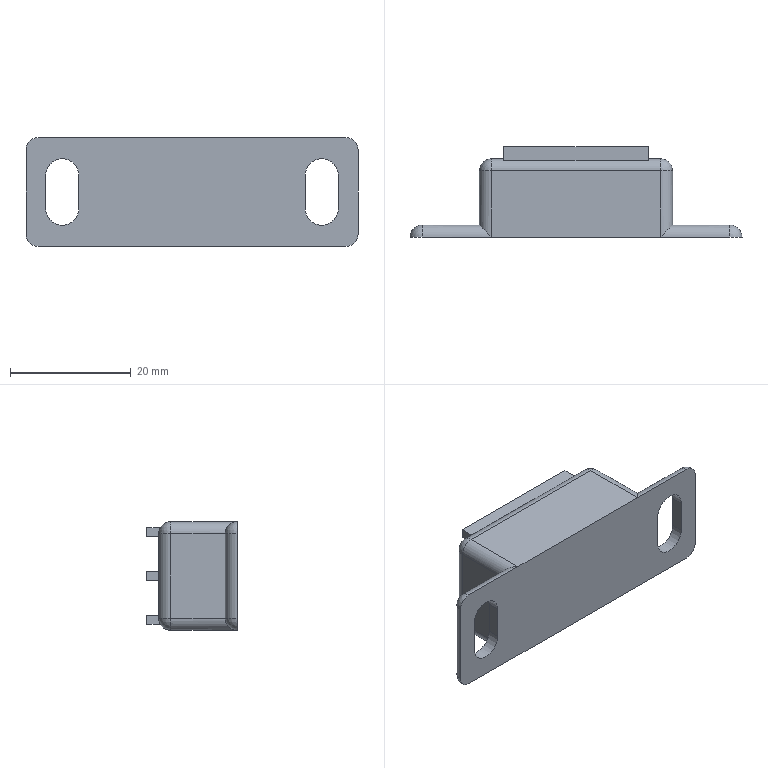Part | NX | features BREP 1 | 1 solid | 53 faces | box 55 x 15 x 18 mm | volume 8127 mm3 | plane 27 | cylinder 18 | sphere 8 | commonest cylinder face diameters 4 x14 5.5 x4
STEP:
#1=CARTESIAN_POINT('',(12.,13.,-6.5));
#2=VERTEX_POINT('',#1);
#3=CARTESIAN_POINT('',(12.,13.,-7.));
#4=VERTEX_POINT('',#3);
#5=CARTESIAN_POINT('',(12.,13.,9.));
#6=DIRECTION('',(0.,0.,-1.));
#7=VECTOR('',#6,1000.);
#8=LINE('',#5,#7);
#9=EDGE_CURVE('',#2,#4,#8,.T.);
#10=ORIENTED_EDGE('',*,*,#9,.F.);
#11=CARTESIAN_POINT('',(-12.,13.,-6.5));
#12=VERTEX_POINT('',#11);
#13=CARTESIAN_POINT('',(16.,13.,-6.5));
#14=DIRECTION('',(1.,0.,0.));
#15=VECTOR('',#14,1000.);
#16=LINE('',#13,#15);
#17=EDGE_CURVE('',#12,#2,#16,.T.);
#18=ORIENTED_EDGE('',*,*,#17,.F.);
#19=CARTESIAN_POINT('',(-12.,13.,-7.));
#20=VERTEX_POINT('',#19);
#21=CARTESIAN_POINT('',(-12.,13.,9.));
#22=DIRECTION('',(0.,0.,1.));
#23=VECTOR('',#22,1000.);
#24=LINE('',#21,#23);
#25=EDGE_CURVE('',#20,#12,#24,.T.);
#26=ORIENTED_EDGE('',*,*,#25,.F.);
#27=CARTESIAN_POINT('',(-14.,13.,-7.));
#28=VERTEX_POINT('',#27);
#29=CARTESIAN_POINT('',(16.,13.,-7.));
#30=DIRECTION('',(-1.,0.,0.));
#31=VECTOR('',#30,1000.);
#32=LINE('',#29,#31);
#33=EDGE_CURVE('',#20,#28,#32,.T.);
#34=ORIENTED_EDGE('',*,*,#33,.T.);
#35=CARTESIAN_POINT('',(-14.,13.,7.));
#36=VERTEX_POINT('',#35);
#37=CARTESIAN_POINT('',(-14.,13.,9.));
#38=DIRECTION('',(0.,0.,1.));
#39=VECTOR('',#38,1000.);
#40=LINE('',#37,#39);
#41=EDGE_CURVE('',#28,#36,#40,.T.);
#42=ORIENTED_EDGE('',*,*,#41,.T.);
#43=CARTESIAN_POINT('',(-12.,13.,7.));
#44=VERTEX_POINT('',#43);
#45=CARTESIAN_POINT('',(16.,13.,7.));
#46=DIRECTION('',(1.,0.,0.));
#47=VECTOR('',#46,1000.);
#48=LINE('',#45,#47);
#49=EDGE_CURVE('',#36,#44,#48,.T.);
#50=ORIENTED_EDGE('',*,*,#49,.T.);
#51=CARTESIAN_POINT('',(-12.,13.,6.5));
#52=VERTEX_POINT('',#51);
#53=CARTESIAN_POINT('',(-12.,13.,9.));
#54=DIRECTION('',(0.,0.,1.));
#55=VECTOR('',#54,1000.);
#56=LINE('',#53,#55);
#57=EDGE_CURVE('',#52,#44,#56,.T.);
#58=ORIENTED_EDGE('',*,*,#57,.F.);
#59=CARTESIAN_POINT('',(12.,13.,6.5));
#60=VERTEX_POINT('',#59);
#61=CARTESIAN_POINT('',(16.,13.,6.5));
#62=DIRECTION('',(-1.,0.,0.));
#63=VECTOR('',#62,1000.);
#64=LINE('',#61,#63);
#65=EDGE_CURVE('',#60,#52,#64,.T.);
#66=ORIENTED_EDGE('',*,*,#65,.F.);
#67=CARTESIAN_POINT('',(12.,13.,7.));
#68=VERTEX_POINT('',#67);
#69=CARTESIAN_POINT('',(12.,13.,9.));
#70=DIRECTION('',(0.,0.,-1.));
#71=VECTOR('',#70,1000.);
#72=LINE('',#69,#71);
#73=EDGE_CURVE('',#68,#60,#72,.T.);
#74=ORIENTED_EDGE('',*,*,#73,.F.);
#75=CARTESIAN_POINT('',(14.,13.,7.));
#76=VERTEX_POINT('',#75);
#77=CARTESIAN_POINT('',(16.,13.,7.));
#78=DIRECTION('',(1.,0.,0.));
#79=VECTOR('',#78,1000.);
#80=LINE('',#77,#79);
#81=EDGE_CURVE('',#68,#76,#80,.T.);
#82=ORIENTED_EDGE('',*,*,#81,.T.);
#83=CARTESIAN_POINT('',(14.,13.,-7.));
#84=VERTEX_POINT('',#83);
#85=CARTESIAN_POINT('',(14.,13.,9.));
#86=DIRECTION('',(0.,0.,-1.));
#87=VECTOR('',#86,1000.);
#88=LINE('',#85,#87);
#89=EDGE_CURVE('',#76,#84,#88,.T.);
#90=ORIENTED_EDGE('',*,*,#89,.T.);
#91=CARTESIAN_POINT('',(16.,13.,-7.));
#92=DIRECTION('',(-1.,0.,0.));
#93=VECTOR('',#92,1000.);
#94=LINE('',#91,#93);
#95=EDGE_CURVE('',#84,#4,#94,.T.);
#96=ORIENTED_EDGE('',*,*,#95,.T.);
#97=EDGE_LOOP('',(#10,#18,#26,#34,#42,#50,#58,#66,#74,#82,#90,#96));
#98=FACE_BOUND('',#97,.T.);
#99=CARTESIAN_POINT('',(12.,13.,0.75));
#100=VERTEX_POINT('',#99);
#101=CARTESIAN_POINT('',(12.,13.,-0.75));
#102=VERTEX_POINT('',#101);
#103=CARTESIAN_POINT('',(12.,13.,9.));
#104=DIRECTION('',(0.,0.,-1.));
#105=VECTOR('',#104,1000.);
#106=LINE('',#103,#105);
#107=EDGE_CURVE('',#100,#102,#106,.T.);
#108=ORIENTED_EDGE('',*,*,#107,.F.);
#109=CARTESIAN_POINT('',(-12.,13.,0.75));
#110=VERTEX_POINT('',#109);
#111=CARTESIAN_POINT('',(16.,13.,0.75));
#112=DIRECTION('',(1.,0.,0.));
#113=VECTOR('',#112,1000.);
#114=LINE('',#111,#113);
#115=EDGE_CURVE('',#110,#100,#114,.T.);
#116=ORIENTED_EDGE('',*,*,#115,.F.);
#117=CARTESIAN_POINT('',(-12.,13.,-0.75));
#118=VERTEX_POINT('',#117);
#119=CARTESIAN_POINT('',(-12.,13.,9.));
#120=DIRECTION('',(0.,0.,1.));
#121=VECTOR('',#120,1000.);
#122=LINE('',#119,#121);
#123=EDGE_CURVE('',#118,#110,#122,.T.);
#124=ORIENTED_EDGE('',*,*,#123,.F.);
#125=CARTESIAN_POINT('',(16.,13.,-0.75));
#126=DIRECTION('',(-1.,0.,0.));
#127=VECTOR('',#126,1000.);
#128=LINE('',#125,#127);
#129=EDGE_CURVE('',#102,#118,#128,.T.);
#130=ORIENTED_EDGE('',*,*,#129,.F.);
#131=EDGE_LOOP('',(#108,#116,#124,#130));
#132=FACE_BOUND('',#131,.T.);
#133=CARTESIAN_POINT('',(16.,13.,9.));
#134=DIRECTION('',(0.,-1.,0.));
#135=DIRECTION('',(0.,0.,-1.));
#136=AXIS2_PLACEMENT_3D('',#133,#134,#135);
#137=PLANE('',#136);
#138=ADVANCED_FACE('',(#98,#132),#137,.F.);
#139=CARTESIAN_POINT('',(-12.,12.732,-8.));
#140=VERTEX_POINT('',#139);
#141=CARTESIAN_POINT('',(12.,12.732,-8.));
#142=VERTEX_POINT('',#141);
#143=CARTESIAN_POINT('',(16.,12.732,-8.));
#144=DIRECTION('',(1.,0.,0.));
#145=VECTOR('',#144,1000.);
#146=LINE('',#143,#145);
#147=EDGE_CURVE('',#140,#142,#146,.T.);
#148=ORIENTED_EDGE('',*,*,#147,.T.);
#149=CARTESIAN_POINT('',(12.,11.,-7.));
#150=DIRECTION('',(1.,0.,0.));
#151=DIRECTION('',(0.,-1.,0.));
#152=AXIS2_PLACEMENT_3D('',#149,#150,#151);
#153=CIRCLE('',#152,2.);
#154=EDGE_CURVE('',#142,#4,#153,.T.);
#155=ORIENTED_EDGE('',*,*,#154,.T.);
#156=ORIENTED_EDGE('',*,*,#95,.F.);
#157=CARTESIAN_POINT('',(14.,11.,-9.));
#158=VERTEX_POINT('',#157);
#159=CARTESIAN_POINT('',(14.,11.,-7.));
#160=DIRECTION('',(1.,0.,0.));
#161=DIRECTION('',(0.,0.,-1.));
#162=AXIS2_PLACEMENT_3D('',#159,#160,#161);
#163=CIRCLE('',#162,2.);
#164=EDGE_CURVE('',#158,#84,#163,.T.);
#165=ORIENTED_EDGE('',*,*,#164,.F.);
#166=CARTESIAN_POINT('',(-14.,11.,-9.));
#167=VERTEX_POINT('',#166);
#168=CARTESIAN_POINT('',(0.,11.,-9.));
#169=DIRECTION('',(1.,0.,0.));
#170=VECTOR('',#169,1000.);
#171=LINE('',#168,#170);
#172=EDGE_CURVE('',#167,#158,#171,.T.);
#173=ORIENTED_EDGE('',*,*,#172,.F.);
#174=CARTESIAN_POINT('',(-14.,11.,-7.));
#175=DIRECTION('',(1.,0.,0.));
#176=DIRECTION('',(0.,0.,1.));
#177=AXIS2_PLACEMENT_3D('',#174,#175,#176);
#178=CIRCLE('',#177,2.);
#179=EDGE_CURVE('',#167,#28,#178,.T.);
#180=ORIENTED_EDGE('',*,*,#179,.T.);
#181=ORIENTED_EDGE('',*,*,#33,.F.);
#182=CARTESIAN_POINT('',(-12.,11.,-7.));
#183=DIRECTION('',(-1.,0.,0.));
#184=DIRECTION('',(0.,1.,0.));
#185=AXIS2_PLACEMENT_3D('',#182,#183,#184);
#186=CIRCLE('',#185,2.);
#187=EDGE_CURVE('',#20,#140,#186,.T.);
#188=ORIENTED_EDGE('',*,*,#187,.T.);
#189=EDGE_LOOP('',(#148,#155,#156,#165,#173,#180,#181,#188));
#190=FACE_BOUND('',#189,.T.);
#191=CARTESIAN_POINT('',(16.,11.,-7.));
#192=DIRECTION('',(-1.,0.,0.));
#193=DIRECTION('',(0.,-1.,0.));
#194=AXIS2_PLACEMENT_3D('',#191,#192,#193);
#195=CYLINDRICAL_SURFACE('',#194,2.);
#196=ADVANCED_FACE('',(#190),#195,.T.);
#197=ORIENTED_EDGE('',*,*,#81,.F.);
#198=CARTESIAN_POINT('',(12.,12.732,8.));
#199=VERTEX_POINT('',#198);
#200=CARTESIAN_POINT('',(12.,11.,7.));
#201=DIRECTION('',(1.,0.,0.));
#202=DIRECTION('',(0.,-1.,0.));
#203=AXIS2_PLACEMENT_3D('',#200,#201,#202);
#204=CIRCLE('',#203,2.);
#205=EDGE_CURVE('',#68,#199,#204,.T.);
#206=ORIENTED_EDGE('',*,*,#205,.T.);
#207=CARTESIAN_POINT('',(-12.,12.732,8.));
#208=VERTEX_POINT('',#207);
#209=CARTESIAN_POINT('',(0.,12.732,8.));
#210=DIRECTION('',(-1.,0.,0.));
#211=VECTOR('',#210,1000.);
#212=LINE('',#209,#211);
#213=EDGE_CURVE('',#199,#208,#212,.T.);
#214=ORIENTED_EDGE('',*,*,#213,.T.);
#215=CARTESIAN_POINT('',(-12.,11.,7.));
#216=DIRECTION('',(-1.,0.,0.));
#217=DIRECTION('',(0.,1.,0.));
#218=AXIS2_PLACEMENT_3D('',#215,#216,#217);
#219=CIRCLE('',#218,2.);
#220=EDGE_CURVE('',#208,#44,#219,.T.);
#221=ORIENTED_EDGE('',*,*,#220,.T.);
#222=ORIENTED_EDGE('',*,*,#49,.F.);
#223=CARTESIAN_POINT('',(-14.,11.,9.));
#224=VERTEX_POINT('',#223);
#225=CARTESIAN_POINT('',(-14.,11.,7.));
#226=DIRECTION('',(1.,0.,0.));
#227=DIRECTION('',(0.,0.,1.));
#228=AXIS2_PLACEMENT_3D('',#225,#226,#227);
#229=CIRCLE('',#228,2.);
#230=EDGE_CURVE('',#36,#224,#229,.T.);
#231=ORIENTED_EDGE('',*,*,#230,.T.);
#232=CARTESIAN_POINT('',(14.,11.,9.));
#233=VERTEX_POINT('',#232);
#234=CARTESIAN_POINT('',(-16.,11.,9.));
#235=DIRECTION('',(-1.,0.,0.));
#236=VECTOR('',#235,1000.);
#237=LINE('',#234,#236);
#238=EDGE_CURVE('',#233,#224,#237,.T.);
#239=ORIENTED_EDGE('',*,*,#238,.F.);
#240=CARTESIAN_POINT('',(14.,11.,7.));
#241=DIRECTION('',(1.,0.,0.));
#242=DIRECTION('',(0.,0.,-1.));
#243=AXIS2_PLACEMENT_3D('',#240,#241,#242);
#244=CIRCLE('',#243,2.);
#245=EDGE_CURVE('',#76,#233,#244,.T.);
#246=ORIENTED_EDGE('',*,*,#245,.F.);
#247=EDGE_LOOP('',(#197,#206,#214,#221,#222,#231,#239,#246));
#248=FACE_BOUND('',#247,.T.);
#249=CARTESIAN_POINT('',(0.,11.,7.));
#250=DIRECTION('',(1.,0.,0.));
#251=DIRECTION('',(0.,1.,0.));
#252=AXIS2_PLACEMENT_3D('',#249,#250,#251);
#253=CYLINDRICAL_SURFACE('',#252,2.);
#254=ADVANCED_FACE('',(#248),#253,.T.);
#255=CARTESIAN_POINT('',(14.,0.,-9.));
#256=VERTEX_POINT('',#255);
#257=CARTESIAN_POINT('',(25.5,0.,-9.));
#258=VERTEX_POINT('',#257);
#259=CARTESIAN_POINT('',(-27.5,0.,-9.));
#260=DIRECTION('',(1.,0.,0.));
#261=VECTOR('',#260,1000.);
#262=LINE('',#259,#261);
#263=EDGE_CURVE('',#256,#258,#262,.T.);
#264=ORIENTED_EDGE('',*,*,#263,.T.);
#265=CARTESIAN_POINT('',(27.5,0.,-7.));
#266=VERTEX_POINT('',#265);
#267=CARTESIAN_POINT('',(25.5,0.,-7.));
#268=DIRECTION('',(0.,-1.,0.));
#269=DIRECTION('',(0.,0.,1.));
#270=AXIS2_PLACEMENT_3D('',#267,#268,#269);
#271=CIRCLE('',#270,2.);
#272=EDGE_CURVE('',#258,#266,#271,.T.);
#273=ORIENTED_EDGE('',*,*,#272,.T.);
#274=CARTESIAN_POINT('',(27.5,0.,7.));
#275=VERTEX_POINT('',#274);
#276=CARTESIAN_POINT('',(27.5,0.,9.));
#277=DIRECTION('',(0.,0.,-1.));
#278=VECTOR('',#277,1000.);
#279=LINE('',#276,#278);
#280=EDGE_CURVE('',#275,#266,#279,.T.);
#281=ORIENTED_EDGE('',*,*,#280,.F.);
#282=CARTESIAN_POINT('',(25.5,0.,9.));
#283=VERTEX_POINT('',#282);
#284=CARTESIAN_POINT('',(25.5,0.,7.));
#285=DIRECTION('',(0.,-1.,0.));
#286=DIRECTION('',(0.,0.,1.));
#287=AXIS2_PLACEMENT_3D('',#284,#285,#286);
#288=CIRCLE('',#287,2.);
#289=EDGE_CURVE('',#275,#283,#288,.T.);
#290=ORIENTED_EDGE('',*,*,#289,.T.);
#291=CARTESIAN_POINT('',(14.,0.,9.));
#292=VERTEX_POINT('',#291);
#293=CARTESIAN_POINT('',(-27.5,0.,9.));
#294=DIRECTION('',(1.,0.,0.));
#295=VECTOR('',#294,1000.);
#296=LINE('',#293,#295);
#297=EDGE_CURVE('',#292,#283,#296,.T.);
#298=ORIENTED_EDGE('',*,*,#297,.F.);
#299=CARTESIAN_POINT('',(-14.,0.,9.));
#300=VERTEX_POINT('',#299);
#301=CARTESIAN_POINT('',(-27.5,0.,9.));
#302=DIRECTION('',(1.,0.,0.));
#303=VECTOR('',#302,1000.);
#304=LINE('',#301,#303);
#305=EDGE_CURVE('',#300,#292,#304,.T.);
#306=ORIENTED_EDGE('',*,*,#305,.F.);
#307=CARTESIAN_POINT('',(-25.5,0.,9.));
#308=VERTEX_POINT('',#307);
#309=CARTESIAN_POINT('',(-27.5,0.,9.));
#310=DIRECTION('',(1.,0.,0.));
#311=VECTOR('',#310,1000.);
#312=LINE('',#309,#311);
#313=EDGE_CURVE('',#308,#300,#312,.T.);
#314=ORIENTED_EDGE('',*,*,#313,.F.);
#315=CARTESIAN_POINT('',(-27.5,0.,7.));
#316=VERTEX_POINT('',#315);
#317=CARTESIAN_POINT('',(-25.5,0.,7.));
#318=DIRECTION('',(0.,-1.,0.));
#319=DIRECTION('',(0.,0.,1.));
#320=AXIS2_PLACEMENT_3D('',#317,#318,#319);
#321=CIRCLE('',#320,2.);
#322=EDGE_CURVE('',#308,#316,#321,.T.);
#323=ORIENTED_EDGE('',*,*,#322,.T.);
#324=CARTESIAN_POINT('',(-27.5,0.,-7.));
#325=VERTEX_POINT('',#324);
#326=CARTESIAN_POINT('',(-27.5,0.,9.));
#327=DIRECTION('',(0.,0.,-1.));
#328=VECTOR('',#327,1000.);
#329=LINE('',#326,#328);
#330=EDGE_CURVE('',#316,#325,#329,.T.);
#331=ORIENTED_EDGE('',*,*,#330,.T.);
#332=CARTESIAN_POINT('',(-25.5,0.,-9.));
#333=VERTEX_POINT('',#332);
#334=CARTESIAN_POINT('',(-25.5,0.,-7.));
#335=DIRECTION('',(0.,-1.,0.));
#336=DIRECTION('',(0.,0.,1.));
#337=AXIS2_PLACEMENT_3D('',#334,#335,#336);
#338=CIRCLE('',#337,2.);
#339=EDGE_CURVE('',#325,#333,#338,.T.);
#340=ORIENTED_EDGE('',*,*,#339,.T.);
#341=CARTESIAN_POINT('',(-14.,0.,-9.));
#342=VERTEX_POINT('',#341);
#343=CARTESIAN_POINT('',(-27.5,0.,-9.));
#344=DIRECTION('',(1.,0.,0.));
#345=VECTOR('',#344,1000.);
#346=LINE('',#343,#345);
#347=EDGE_CURVE('',#333,#342,#346,.T.);
#348=ORIENTED_EDGE('',*,*,#347,.T.);
#349=CARTESIAN_POINT('',(-27.5,0.,-9.));
#350=DIRECTION('',(1.,0.,0.));
#351=VECTOR('',#350,1000.);
#352=LINE('',#349,#351);
#353=EDGE_CURVE('',#342,#256,#352,.T.);
#354=ORIENTED_EDGE('',*,*,#353,.T.);
#355=EDGE_LOOP('',(#264,#273,#281,#290,#298,#306,#314,#323,#331,#340,#348,#354));
#356=FACE_BOUND('',#355,.T.);
#357=CARTESIAN_POINT('',(24.25,0.,2.75));
#358=VERTEX_POINT('',#357);
#359=CARTESIAN_POINT('',(24.25,0.,-2.75));
#360=VERTEX_POINT('',#359);
#361=CARTESIAN_POINT('',(24.25,0.,-2.75));
#362=DIRECTION('',(0.,0.,-1.));
#363=VECTOR('',#362,1000.);
#364=LINE('',#361,#363);
#365=EDGE_CURVE('',#358,#360,#364,.T.);
#366=ORIENTED_EDGE('',*,*,#365,.T.);
#367=CARTESIAN_POINT('',(18.75,0.,-2.75));
#368=VERTEX_POINT('',#367);
#369=CARTESIAN_POINT('',(21.5,0.,-2.75));
#370=DIRECTION('',(0.,1.,0.));
#371=DIRECTION('',(-1.,0.,0.));
#372=AXIS2_PLACEMENT_3D('',#369,#370,#371);
#373=CIRCLE('',#372,2.75);
#374=EDGE_CURVE('',#360,#368,#373,.T.);
#375=ORIENTED_EDGE('',*,*,#374,.T.);
#376=CARTESIAN_POINT('',(18.75,0.,2.75));
#377=VERTEX_POINT('',#376);
#378=CARTESIAN_POINT('',(18.75,0.,-2.75));
#379=DIRECTION('',(0.,0.,1.));
#380=VECTOR('',#379,1000.);
#381=LINE('',#378,#380);
#382=EDGE_CURVE('',#368,#377,#381,.T.);
#383=ORIENTED_EDGE('',*,*,#382,.T.);
#384=CARTESIAN_POINT('',(21.5,0.,2.75));
#385=DIRECTION('',(0.,1.,0.));
#386=DIRECTION('',(-1.,0.,0.));
#387=AXIS2_PLACEMENT_3D('',#384,#385,#386);
#388=CIRCLE('',#387,2.75);
#389=EDGE_CURVE('',#377,#358,#388,.T.);
#390=ORIENTED_EDGE('',*,*,#389,.T.);
#391=EDGE_LOOP('',(#366,#375,#383,#390));
#392=FACE_BOUND('',#391,.T.);
#393=CARTESIAN_POINT('',(-18.75,0.,2.75));
#394=VERTEX_POINT('',#393);
#395=CARTESIAN_POINT('',(-18.75,0.,-2.75));
#396=VERTEX_POINT('',#395);
#397=CARTESIAN_POINT('',(-18.75,0.,-2.75));
#398=DIRECTION('',(0.,0.,-1.));
#399=VECTOR('',#398,1000.);
#400=LINE('',#397,#399);
#401=EDGE_CURVE('',#394,#396,#400,.T.);
#402=ORIENTED_EDGE('',*,*,#401,.T.);
#403=CARTESIAN_POINT('',(-24.25,0.,-2.75));
#404=VERTEX_POINT('',#403);
#405=CARTESIAN_POINT('',(-21.5,0.,-2.75));
#406=DIRECTION('',(0.,1.,0.));
#407=DIRECTION('',(-1.,0.,0.));
#408=AXIS2_PLACEMENT_3D('',#405,#406,#407);
#409=CIRCLE('',#408,2.75);
#410=EDGE_CURVE('',#396,#404,#409,.T.);
#411=ORIENTED_EDGE('',*,*,#410,.T.);
#412=CARTESIAN_POINT('',(-24.25,0.,2.75));
#413=VERTEX_POINT('',#412);
#414=CARTESIAN_POINT('',(-24.25,0.,-2.75));
#415=DIRECTION('',(0.,0.,1.));
#416=VECTOR('',#415,1000.);
#417=LINE('',#414,#416);
#418=EDGE_CURVE('',#404,#413,#417,.T.);
#419=ORIENTED_EDGE('',*,*,#418,.T.);
#420=CARTESIAN_POINT('',(-21.5,0.,2.75));
#421=DIRECTION('',(0.,1.,0.));
#422=DIRECTION('',(-1.,0.,0.));
#423=AXIS2_PLACEMENT_3D('',#420,#421,#422);
#424=CIRCLE('',#423,2.75);
#425=EDGE_CURVE('',#413,#394,#424,.T.);
#426=ORIENTED_EDGE('',*,*,#425,.T.);
#427=EDGE_LOOP('',(#402,#411,#419,#426));
#428=FACE_BOUND('',#427,.T.);
#429=CARTESIAN_POINT('',(-27.5,0.,9.));
#430=DIRECTION('',(0.,1.,0.));
#431=DIRECTION('',(1.,0.,0.));
#432=AXIS2_PLACEMENT_3D('',#429,#430,#431);
#433=PLANE('',#432);
#434=ADVANCED_FACE('',(#356,#392,#428),#433,.F.);
#435=CARTESIAN_POINT('',(25.5,2.,7.));
#436=VERTEX_POINT('',#435);
#437=CARTESIAN_POINT('',(25.5,2.,-7.));
#438=VERTEX_POINT('',#437);
#439=CARTESIAN_POINT('',(25.5,2.,9.));
#440=DIRECTION('',(0.,0.,-1.));
#441=VECTOR('',#440,1000.);
#442=LINE('',#439,#441);
#443=EDGE_CURVE('',#436,#438,#442,.T.);
#444=ORIENTED_EDGE('',*,*,#443,.T.);
#445=CARTESIAN_POINT('',(16.,2.,-7.));
#446=VERTEX_POINT('',#445);
#447=CARTESIAN_POINT('',(27.5,2.,-7.));
#448=DIRECTION('',(-1.,0.,0.));
#449=VECTOR('',#448,1000.);
#450=LINE('',#447,#449);
#451=EDGE_CURVE('',#438,#446,#450,.T.);
#452=ORIENTED_EDGE('',*,*,#451,.T.);
#453=CARTESIAN_POINT('',(16.,2.,7.));
#454=VERTEX_POINT('',#453);
#455=CARTESIAN_POINT('',(16.,2.,9.));
#456=DIRECTION('',(0.,0.,-1.));
#457=VECTOR('',#456,1000.);
#458=LINE('',#455,#457);
#459=EDGE_CURVE('',#454,#446,#458,.T.);
#460=ORIENTED_EDGE('',*,*,#459,.F.);
#461=CARTESIAN_POINT('',(27.5,2.,7.));
#462=DIRECTION('',(1.,0.,0.));
#463=VECTOR('',#462,1000.);
#464=LINE('',#461,#463);
#465=EDGE_CURVE('',#454,#436,#464,.T.);
#466=ORIENTED_EDGE('',*,*,#465,.T.);
#467=EDGE_LOOP('',(#444,#452,#460,#466));
#468=FACE_BOUND('',#467,.T.);
#469=CARTESIAN_POINT('',(18.75,2.,-2.75));
#470=VERTEX_POINT('',#469);
#471=CARTESIAN_POINT('',(18.75,2.,2.75));
#472=VERTEX_POINT('',#471);
#473=CARTESIAN_POINT('',(18.75,2.,-2.75));
#474=DIRECTION('',(0.,0.,1.));
#475=VECTOR('',#474,1000.);
#476=LINE('',#473,#475);
#477=EDGE_CURVE('',#470,#472,#476,.T.);
#478=ORIENTED_EDGE('',*,*,#477,.F.);
#479=CARTESIAN_POINT('',(24.25,2.,-2.75));
#480=VERTEX_POINT('',#479);
#481=CARTESIAN_POINT('',(21.5,2.,-2.75));
#482=DIRECTION('',(0.,1.,0.));
#483=DIRECTION('',(-1.,0.,0.));
#484=AXIS2_PLACEMENT_3D('',#481,#482,#483);
#485=CIRCLE('',#484,2.75);
#486=EDGE_CURVE('',#480,#470,#485,.T.);
#487=ORIENTED_EDGE('',*,*,#486,.F.);
#488=CARTESIAN_POINT('',(24.25,2.,2.75));
#489=VERTEX_POINT('',#488);
#490=CARTESIAN_POINT('',(24.25,2.,-2.75));
#491=DIRECTION('',(0.,0.,-1.));
#492=VECTOR('',#491,1000.);
#493=LINE('',#490,#492);
#494=EDGE_CURVE('',#489,#480,#493,.T.);
#495=ORIENTED_EDGE('',*,*,#494,.F.);
#496=CARTESIAN_POINT('',(21.5,2.,2.75));
#497=DIRECTION('',(0.,1.,0.));
#498=DIRECTION('',(-1.,0.,0.));
#499=AXIS2_PLACEMENT_3D('',#496,#497,#498);
#500=CIRCLE('',#499,2.75);
#501=EDGE_CURVE('',#472,#489,#500,.T.);
#502=ORIENTED_EDGE('',*,*,#501,.F.);
#503=EDGE_LOOP('',(#478,#487,#495,#502));
#504=FACE_BOUND('',#503,.T.);
#505=CARTESIAN_POINT('',(27.5,2.,9.));
#506=DIRECTION('',(0.,-1.,0.));
#507=DIRECTION('',(-1.,0.,0.));
#508=AXIS2_PLACEMENT_3D('',#505,#506,#507);
#509=PLANE('',#508);
#510=ADVANCED_FACE('',(#468,#504),#509,.F.);
#511=ORIENTED_EDGE('',*,*,#459,.T.);
#512=CARTESIAN_POINT('',(16.,11.,-7.));
#513=VERTEX_POINT('',#512);
#514=CARTESIAN_POINT('',(16.,2.,-7.));
#515=DIRECTION('',(0.,1.,0.));
#516=VECTOR('',#515,1000.);
#517=LINE('',#514,#516);
#518=EDGE_CURVE('',#446,#513,#517,.T.);
#519=ORIENTED_EDGE('',*,*,#518,.T.);
#520=CARTESIAN_POINT('',(16.,11.,7.));
#521=VERTEX_POINT('',#520);
#522=CARTESIAN_POINT('',(16.,11.,9.));
#523=DIRECTION('',(0.,0.,1.));
#524=VECTOR('',#523,1000.);
#525=LINE('',#522,#524);
#526=EDGE_CURVE('',#513,#521,#525,.T.);
#527=ORIENTED_EDGE('',*,*,#526,.T.);
#528=CARTESIAN_POINT('',(16.,2.,7.));
#529=DIRECTION('',(0.,-1.,0.));
#530=VECTOR('',#529,1000.);
#531=LINE('',#528,#530);
#532=EDGE_CURVE('',#521,#454,#531,.T.);
#533=ORIENTED_EDGE('',*,*,#532,.T.);
#534=EDGE_LOOP('',(#511,#519,#527,#533));
#535=FACE_BOUND('',#534,.T.);
#536=CARTESIAN_POINT('',(16.,2.,9.));
#537=DIRECTION('',(-1.,0.,0.));
#538=DIRECTION('',(0.,0.,1.));
#539=AXIS2_PLACEMENT_3D('',#536,#537,#538);
#540=PLANE('',#539);
#541=ADVANCED_FACE('',(#535),#540,.F.);
#542=CARTESIAN_POINT('',(-16.,11.,7.));
#543=VERTEX_POINT('',#542);
#544=CARTESIAN_POINT('',(-16.,11.,-7.));
#545=VERTEX_POINT('',#544);
#546=CARTESIAN_POINT('',(-16.,11.,9.));
#547=DIRECTION('',(0.,0.,-1.));
#548=VECTOR('',#547,1000.);
#549=LINE('',#546,#548);
#550=EDGE_CURVE('',#543,#545,#549,.T.);
#551=ORIENTED_EDGE('',*,*,#550,.T.);
#552=CARTESIAN_POINT('',(-16.,2.,-7.));
#553=VERTEX_POINT('',#552);
#554=CARTESIAN_POINT('',(-16.,13.,-7.));
#555=DIRECTION('',(0.,-1.,0.));
#556=VECTOR('',#555,1000.);
#557=LINE('',#554,#556);
#558=EDGE_CURVE('',#545,#553,#557,.T.);
#559=ORIENTED_EDGE('',*,*,#558,.T.);
#560=CARTESIAN_POINT('',(-16.,2.,7.));
#561=VERTEX_POINT('',#560);
#562=CARTESIAN_POINT('',(-16.,2.,9.));
#563=DIRECTION('',(0.,0.,-1.));
#564=VECTOR('',#563,1000.);
#565=LINE('',#562,#564);
#566=EDGE_CURVE('',#561,#553,#565,.T.);
#567=ORIENTED_EDGE('',*,*,#566,.F.);
#568=CARTESIAN_POINT('',(-16.,13.,7.));
#569=DIRECTION('',(0.,1.,0.));
#570=VECTOR('',#569,1000.);
#571=LINE('',#568,#570);
#572=EDGE_CURVE('',#561,#543,#571,.T.);
#573=ORIENTED_EDGE('',*,*,#572,.T.);
#574=EDGE_LOOP('',(#551,#559,#567,#573));
#575=FACE_BOUND('',#574,.T.);
#576=CARTESIAN_POINT('',(-16.,13.,9.));
#577=DIRECTION('',(1.,0.,0.));
#578=DIRECTION('',(0.,1.,0.));
#579=AXIS2_PLACEMENT_3D('',#576,#577,#578);
#580=PLANE('',#579);
#581=ADVANCED_FACE('',(#575),#580,.F.);
#582=ORIENTED_EDGE('',*,*,#566,.T.);
#583=CARTESIAN_POINT('',(-25.5,2.,-7.));
#584=VERTEX_POINT('',#583);
#585=CARTESIAN_POINT('',(-16.,2.,-7.));
#586=DIRECTION('',(-1.,0.,0.));
#587=VECTOR('',#586,1000.);
#588=LINE('',#585,#587);
#589=EDGE_CURVE('',#553,#584,#588,.T.);
#590=ORIENTED_EDGE('',*,*,#589,.T.);
#591=CARTESIAN_POINT('',(-25.5,2.,7.));
#592=VERTEX_POINT('',#591);
#593=CARTESIAN_POINT('',(-25.5,2.,9.));
#594=DIRECTION('',(0.,0.,1.));
#595=VECTOR('',#594,1000.);
#596=LINE('',#593,#595);
#597=EDGE_CURVE('',#584,#592,#596,.T.);
#598=ORIENTED_EDGE('',*,*,#597,.T.);
#599=CARTESIAN_POINT('',(-16.,2.,7.));
#600=DIRECTION('',(1.,0.,0.));
#601=VECTOR('',#600,1000.);
#602=LINE('',#599,#601);
#603=EDGE_CURVE('',#592,#561,#602,.T.);
#604=ORIENTED_EDGE('',*,*,#603,.T.);
#605=EDGE_LOOP('',(#582,#590,#598,#604));
#606=FACE_BOUND('',#605,.T.);
#607=CARTESIAN_POINT('',(-24.25,2.,-2.75));
#608=VERTEX_POINT('',#607);
#609=CARTESIAN_POINT('',(-24.25,2.,2.75));
#610=VERTEX_POINT('',#609);
#611=CARTESIAN_POINT('',(-24.25,2.,-2.75));
#612=DIRECTION('',(0.,0.,1.));
#613=VECTOR('',#612,1000.);
#614=LINE('',#611,#613);
#615=EDGE_CURVE('',#608,#610,#614,.T.);
#616=ORIENTED_EDGE('',*,*,#615,.F.);
#617=CARTESIAN_POINT('',(-18.75,2.,-2.75));
#618=VERTEX_POINT('',#617);
#619=CARTESIAN_POINT('',(-21.5,2.,-2.75));
#620=DIRECTION('',(0.,1.,0.));
#621=DIRECTION('',(-1.,0.,0.));
#622=AXIS2_PLACEMENT_3D('',#619,#620,#621);
#623=CIRCLE('',#622,2.75);
#624=EDGE_CURVE('',#618,#608,#623,.T.);
#625=ORIENTED_EDGE('',*,*,#624,.F.);
#626=CARTESIAN_POINT('',(-18.75,2.,2.75));
#627=VERTEX_POINT('',#626);
#628=CARTESIAN_POINT('',(-18.75,2.,-2.75));
#629=DIRECTION('',(0.,0.,-1.));
#630=VECTOR('',#629,1000.);
#631=LINE('',#628,#630);
#632=EDGE_CURVE('',#627,#618,#631,.T.);
#633=ORIENTED_EDGE('',*,*,#632,.F.);
#634=CARTESIAN_POINT('',(-21.5,2.,2.75));
#635=DIRECTION('',(0.,1.,0.));
#636=DIRECTION('',(-1.,0.,0.));
#637=AXIS2_PLACEMENT_3D('',#634,#635,#636);
#638=CIRCLE('',#637,2.75);
#639=EDGE_CURVE('',#610,#627,#638,.T.);
#640=ORIENTED_EDGE('',*,*,#639,.F.);
#641=EDGE_LOOP('',(#616,#625,#633,#640));
#642=FACE_BOUND('',#641,.T.);
#643=CARTESIAN_POINT('',(-16.,2.,9.));
#644=DIRECTION('',(0.,-1.,0.));
#645=DIRECTION('',(0.,0.,-1.));
#646=AXIS2_PLACEMENT_3D('',#643,#644,#645);
#647=PLANE('',#646);
#648=ADVANCED_FACE('',(#606,#642),#647,.F.);
#649=ORIENTED_EDGE('',*,*,#238,.T.);
#650=CARTESIAN_POINT('',(-14.,2.,9.));
#651=DIRECTION('',(0.,-1.,0.));
#652=VECTOR('',#651,1000.);
#653=LINE('',#650,#652);
#654=EDGE_CURVE('',#224,#300,#653,.T.);
#655=ORIENTED_EDGE('',*,*,#654,.T.);
#656=ORIENTED_EDGE('',*,*,#305,.T.);
#657=CARTESIAN_POINT('',(14.,13.,9.));
#658=DIRECTION('',(0.,1.,0.));
#659=VECTOR('',#658,1000.);
#660=LINE('',#657,#659);
#661=EDGE_CURVE('',#292,#233,#660,.T.);
#662=ORIENTED_EDGE('',*,*,#661,.T.);
#663=EDGE_LOOP('',(#649,#655,#656,#662));
#664=FACE_BOUND('',#663,.T.);
#665=CARTESIAN_POINT('',(0.,0.,9.));
#666=DIRECTION('',(0.,0.,1.));
#667=DIRECTION('',(1.,0.,0.));
#668=AXIS2_PLACEMENT_3D('',#665,#666,#667);
#669=PLANE('',#668);
#670=ADVANCED_FACE('',(#664),#669,.T.);
#671=ORIENTED_EDGE('',*,*,#353,.F.);
#672=CARTESIAN_POINT('',(-14.,0.,-9.));
#673=DIRECTION('',(0.,1.,0.));
#674=VECTOR('',#673,1000.);
#675=LINE('',#672,#674);
#676=EDGE_CURVE('',#342,#167,#675,.T.);
#677=ORIENTED_EDGE('',*,*,#676,.T.);
#678=ORIENTED_EDGE('',*,*,#172,.T.);
#679=CARTESIAN_POINT('',(14.,0.,-9.));
#680=DIRECTION('',(0.,-1.,0.));
#681=VECTOR('',#680,1000.);
#682=LINE('',#679,#681);
#683=EDGE_CURVE('',#158,#256,#682,.T.);
#684=ORIENTED_EDGE('',*,*,#683,.T.);
#685=EDGE_LOOP('',(#671,#677,#678,#684));
#686=FACE_BOUND('',#685,.T.);
#687=CARTESIAN_POINT('',(0.,0.,-9.));
#688=DIRECTION('',(0.,0.,1.));
#689=DIRECTION('',(1.,0.,0.));
#690=AXIS2_PLACEMENT_3D('',#687,#688,#689);
#691=PLANE('',#690);
#692=ADVANCED_FACE('',(#686),#691,.F.);
#693=CARTESIAN_POINT('',(-25.5,0.,7.));
#694=DIRECTION('',(0.,0.,-1.));
#695=DIRECTION('',(1.,0.,0.));
#696=AXIS2_PLACEMENT_3D('',#693,#694,#695);
#697=CIRCLE('',#696,2.);
#698=EDGE_CURVE('',#316,#592,#697,.T.);
#699=ORIENTED_EDGE('',*,*,#698,.F.);
#700=ORIENTED_EDGE('',*,*,#322,.F.);
#701=CARTESIAN_POINT('',(-25.5,0.,7.));
#702=DIRECTION('',(1.,0.,0.));
#703=DIRECTION('',(0.,0.,1.));
#704=AXIS2_PLACEMENT_3D('',#701,#702,#703);
#705=CIRCLE('',#704,2.);
#706=EDGE_CURVE('',#592,#308,#705,.T.);
#707=ORIENTED_EDGE('',*,*,#706,.F.);
#708=EDGE_LOOP('',(#699,#700,#707));
#709=FACE_BOUND('',#708,.T.);
#710=CARTESIAN_POINT('',(-25.5,0.,7.));
#711=DIRECTION('',(0.,0.,-1.));
#712=DIRECTION('',(1.,0.,0.));
#713=AXIS2_PLACEMENT_3D('',#710,#711,#712);
#714=SPHERICAL_SURFACE('',#713,2.);
#715=ADVANCED_FACE('',(#709),#714,.T.);
#716=ORIENTED_EDGE('',*,*,#706,.T.);
#717=ORIENTED_EDGE('',*,*,#313,.T.);
#718=CARTESIAN_POINT('',(-16.,2.,7.));
#719=CARTESIAN_POINT('',(-16.,2.,8.172));
#720=CARTESIAN_POINT('',(-15.172,1.172,9.));
#721=CARTESIAN_POINT('',(-14.,0.,9.));
#722=(BOUNDED_CURVE()B_SPLINE_CURVE(3,(#718,#719,#720,#721),.UNSPECIFIED.,.F.,.F.)B_SPLINE_CURVE_WITH_KNOTS((4,4),(3.142,4.712),.UNSPECIFIED.)CURVE()GEOMETRIC_REPRESENTATION_ITEM()RATIONAL_B_SPLINE_CURVE((1.,0.8047,0.8047,1.))REPRESENTATION_ITEM(''));
#723=EDGE_CURVE('',#561,#300,#722,.T.);
#724=ORIENTED_EDGE('',*,*,#723,.F.);
#725=ORIENTED_EDGE('',*,*,#603,.F.);
#726=EDGE_LOOP('',(#716,#717,#724,#725));
#727=FACE_BOUND('',#726,.T.);
#728=CARTESIAN_POINT('',(0.,0.,7.));
#729=DIRECTION('',(1.,0.,0.));
#730=DIRECTION('',(0.,1.,0.));
#731=AXIS2_PLACEMENT_3D('',#728,#729,#730);
#732=CYLINDRICAL_SURFACE('',#731,2.);
#733=ADVANCED_FACE('',(#727),#732,.T.);
#734=ORIENTED_EDGE('',*,*,#698,.T.);
#735=ORIENTED_EDGE('',*,*,#597,.F.);
#736=CARTESIAN_POINT('',(-25.5,0.,-7.));
#737=DIRECTION('',(0.,0.,-1.));
#738=DIRECTION('',(-1.,0.,0.));
#739=AXIS2_PLACEMENT_3D('',#736,#737,#738);
#740=CIRCLE('',#739,2.);
#741=EDGE_CURVE('',#325,#584,#740,.T.);
#742=ORIENTED_EDGE('',*,*,#741,.F.);
#743=ORIENTED_EDGE('',*,*,#330,.F.);
#744=EDGE_LOOP('',(#734,#735,#742,#743));
#745=FACE_BOUND('',#744,.T.);
#746=CARTESIAN_POINT('',(-25.5,0.,9.));
#747=DIRECTION('',(0.,0.,-1.));
#748=DIRECTION('',(-1.,0.,0.));
#749=AXIS2_PLACEMENT_3D('',#746,#747,#748);
#750=CYLINDRICAL_SURFACE('',#749,2.);
#751=ADVANCED_FACE('',(#745),#750,.T.);
#752=ORIENTED_EDGE('',*,*,#723,.T.);
#753=ORIENTED_EDGE('',*,*,#654,.F.);
#754=CARTESIAN_POINT('',(-14.,11.,7.));
#755=DIRECTION('',(0.,1.,0.));
#756=DIRECTION('',(0.,0.,1.));
#757=AXIS2_PLACEMENT_3D('',#754,#755,#756);
#758=CIRCLE('',#757,2.);
#759=EDGE_CURVE('',#543,#224,#758,.T.);
#760=ORIENTED_EDGE('',*,*,#759,.F.);
#761=ORIENTED_EDGE('',*,*,#572,.F.);
#762=EDGE_LOOP('',(#752,#753,#760,#761));
#763=FACE_BOUND('',#762,.T.);
#764=CARTESIAN_POINT('',(-14.,0.,7.));
#765=DIRECTION('',(0.,1.,0.));
#766=DIRECTION('',(0.,0.,1.));
#767=AXIS2_PLACEMENT_3D('',#764,#765,#766);
#768=CYLINDRICAL_SURFACE('',#767,2.);
#769=ADVANCED_FACE('',(#763),#768,.T.);
#770=ORIENTED_EDGE('',*,*,#339,.F.);
#771=ORIENTED_EDGE('',*,*,#741,.T.);
#772=CARTESIAN_POINT('',(-25.5,0.,-7.));
#773=DIRECTION('',(1.,0.,0.));
#774=DIRECTION('',(0.,0.,1.));
#775=AXIS2_PLACEMENT_3D('',#772,#773,#774);
#776=CIRCLE('',#775,2.);
#777=EDGE_CURVE('',#333,#584,#776,.T.);
#778=ORIENTED_EDGE('',*,*,#777,.F.);
#779=EDGE_LOOP('',(#770,#771,#778));
#780=FACE_BOUND('',#779,.T.);
#781=CARTESIAN_POINT('',(-25.5,0.,-7.));
#782=DIRECTION('',(0.,0.,-1.));
#783=DIRECTION('',(1.,0.,0.));
#784=AXIS2_PLACEMENT_3D('',#781,#782,#783);
#785=SPHERICAL_SURFACE('',#784,2.);
#786=ADVANCED_FACE('',(#780),#785,.T.);
#787=CARTESIAN_POINT('',(-14.,11.,7.));
#788=DIRECTION('',(0.,0.,-1.));
#789=DIRECTION('',(1.,0.,0.));
#790=AXIS2_PLACEMENT_3D('',#787,#788,#789);
#791=CIRCLE('',#790,2.);
#792=EDGE_CURVE('',#543,#36,#791,.T.);
#793=ORIENTED_EDGE('',*,*,#792,.F.);
#794=ORIENTED_EDGE('',*,*,#759,.T.);
#795=ORIENTED_EDGE('',*,*,#230,.F.);
#796=EDGE_LOOP('',(#793,#794,#795));
#797=FACE_BOUND('',#796,.T.);
#798=CARTESIAN_POINT('',(-14.,11.,7.));
#799=DIRECTION('',(0.,0.,-1.));
#800=DIRECTION('',(1.,0.,0.));
#801=AXIS2_PLACEMENT_3D('',#798,#799,#800);
#802=SPHERICAL_SURFACE('',#801,2.);
#803=ADVANCED_FACE('',(#797),#802,.T.);
#804=ORIENTED_EDGE('',*,*,#777,.T.);
#805=ORIENTED_EDGE('',*,*,#589,.F.);
#806=CARTESIAN_POINT('',(-14.,0.,-9.));
#807=CARTESIAN_POINT('',(-15.172,1.172,-9.));
#808=CARTESIAN_POINT('',(-16.,2.,-8.172));
#809=CARTESIAN_POINT('',(-16.,2.,-7.));
#810=(BOUNDED_CURVE()B_SPLINE_CURVE(3,(#806,#807,#808,#809),.UNSPECIFIED.,.F.,.F.)B_SPLINE_CURVE_WITH_KNOTS((4,4),(4.712,6.283),.UNSPECIFIED.)CURVE()GEOMETRIC_REPRESENTATION_ITEM()RATIONAL_B_SPLINE_CURVE((1.,0.8047,0.8047,1.))REPRESENTATION_ITEM(''));
#811=EDGE_CURVE('',#342,#553,#810,.T.);
#812=ORIENTED_EDGE('',*,*,#811,.F.);
#813=ORIENTED_EDGE('',*,*,#347,.F.);
#814=EDGE_LOOP('',(#804,#805,#812,#813));
#815=FACE_BOUND('',#814,.T.);
#816=CARTESIAN_POINT('',(-16.,0.,-7.));
#817=DIRECTION('',(-1.,0.,0.));
#818=DIRECTION('',(0.,-1.,0.));
#819=AXIS2_PLACEMENT_3D('',#816,#817,#818);
#820=CYLINDRICAL_SURFACE('',#819,2.);
#821=ADVANCED_FACE('',(#815),#820,.T.);
#822=ORIENTED_EDGE('',*,*,#792,.T.);
#823=ORIENTED_EDGE('',*,*,#41,.F.);
#824=CARTESIAN_POINT('',(-14.,11.,-7.));
#825=DIRECTION('',(0.,0.,-1.));
#826=DIRECTION('',(-1.,0.,0.));
#827=AXIS2_PLACEMENT_3D('',#824,#825,#826);
#828=CIRCLE('',#827,2.);
#829=EDGE_CURVE('',#545,#28,#828,.T.);
#830=ORIENTED_EDGE('',*,*,#829,.F.);
#831=ORIENTED_EDGE('',*,*,#550,.F.);
#832=EDGE_LOOP('',(#822,#823,#830,#831));
#833=FACE_BOUND('',#832,.T.);
#834=CARTESIAN_POINT('',(-14.,11.,9.));
#835=DIRECTION('',(0.,0.,-1.));
#836=DIRECTION('',(-1.,0.,0.));
#837=AXIS2_PLACEMENT_3D('',#834,#835,#836);
#838=CYLINDRICAL_SURFACE('',#837,2.);
#839=ADVANCED_FACE('',(#833),#838,.T.);
#840=ORIENTED_EDGE('',*,*,#811,.T.);
#841=ORIENTED_EDGE('',*,*,#558,.F.);
#842=CARTESIAN_POINT('',(-14.,11.,-7.));
#843=DIRECTION('',(0.,1.,0.));
#844=DIRECTION('',(0.,0.,1.));
#845=AXIS2_PLACEMENT_3D('',#842,#843,#844);
#846=CIRCLE('',#845,2.);
#847=EDGE_CURVE('',#167,#545,#846,.T.);
#848=ORIENTED_EDGE('',*,*,#847,.F.);
#849=ORIENTED_EDGE('',*,*,#676,.F.);
#850=EDGE_LOOP('',(#840,#841,#848,#849));
#851=FACE_BOUND('',#850,.T.);
#852=CARTESIAN_POINT('',(-14.,13.,-7.));
#853=DIRECTION('',(0.,-1.,0.));
#854=DIRECTION('',(0.,0.,-1.));
#855=AXIS2_PLACEMENT_3D('',#852,#853,#854);
#856=CYLINDRICAL_SURFACE('',#855,2.);
#857=ADVANCED_FACE('',(#851),#856,.T.);
#858=CARTESIAN_POINT('',(14.,11.,7.));
#859=DIRECTION('',(0.,0.,-1.));
#860=DIRECTION('',(1.,0.,0.));
#861=AXIS2_PLACEMENT_3D('',#858,#859,#860);
#862=CIRCLE('',#861,2.);
#863=EDGE_CURVE('',#76,#521,#862,.T.);
#864=ORIENTED_EDGE('',*,*,#863,.F.);
#865=ORIENTED_EDGE('',*,*,#245,.T.);
#866=CARTESIAN_POINT('',(14.,11.,7.));
#867=DIRECTION('',(0.,-1.,0.));
#868=DIRECTION('',(0.,0.,1.));
#869=AXIS2_PLACEMENT_3D('',#866,#867,#868);
#870=CIRCLE('',#869,2.);
#871=EDGE_CURVE('',#521,#233,#870,.T.);
#872=ORIENTED_EDGE('',*,*,#871,.F.);
#873=EDGE_LOOP('',(#864,#865,#872));
#874=FACE_BOUND('',#873,.T.);
#875=CARTESIAN_POINT('',(14.,11.,7.));
#876=DIRECTION('',(0.,0.,-1.));
#877=DIRECTION('',(1.,0.,0.));
#878=AXIS2_PLACEMENT_3D('',#875,#876,#877);
#879=SPHERICAL_SURFACE('',#878,2.);
#880=ADVANCED_FACE('',(#874),#879,.T.);
#881=ORIENTED_EDGE('',*,*,#847,.T.);
#882=ORIENTED_EDGE('',*,*,#829,.T.);
#883=ORIENTED_EDGE('',*,*,#179,.F.);
#884=EDGE_LOOP('',(#881,#882,#883));
#885=FACE_BOUND('',#884,.T.);
#886=CARTESIAN_POINT('',(-14.,11.,-7.));
#887=DIRECTION('',(0.,0.,-1.));
#888=DIRECTION('',(1.,0.,0.));
#889=AXIS2_PLACEMENT_3D('',#886,#887,#888);
#890=SPHERICAL_SURFACE('',#889,2.);
#891=ADVANCED_FACE('',(#885),#890,.T.);
#892=ORIENTED_EDGE('',*,*,#871,.T.);
#893=ORIENTED_EDGE('',*,*,#661,.F.);
#894=CARTESIAN_POINT('',(16.,2.,7.));
#895=CARTESIAN_POINT('',(16.,2.,8.172));
#896=CARTESIAN_POINT('',(15.172,1.172,9.));
#897=CARTESIAN_POINT('',(14.,0.,9.));
#898=(BOUNDED_CURVE()B_SPLINE_CURVE(3,(#894,#895,#896,#897),.UNSPECIFIED.,.F.,.F.)B_SPLINE_CURVE_WITH_KNOTS((4,4),(0.,1.571),.UNSPECIFIED.)CURVE()GEOMETRIC_REPRESENTATION_ITEM()RATIONAL_B_SPLINE_CURVE((1.,0.8047,0.8047,1.))REPRESENTATION_ITEM(''));
#899=EDGE_CURVE('',#454,#292,#898,.T.);
#900=ORIENTED_EDGE('',*,*,#899,.F.);
#901=ORIENTED_EDGE('',*,*,#532,.F.);
#902=EDGE_LOOP('',(#892,#893,#900,#901));
#903=FACE_BOUND('',#902,.T.);
#904=CARTESIAN_POINT('',(14.,0.,7.));
#905=DIRECTION('',(0.,-1.,0.));
#906=DIRECTION('',(0.,0.,-1.));
#907=AXIS2_PLACEMENT_3D('',#904,#905,#906);
#908=CYLINDRICAL_SURFACE('',#907,2.);
#909=ADVANCED_FACE('',(#903),#908,.T.);
#910=ORIENTED_EDGE('',*,*,#863,.T.);
#911=ORIENTED_EDGE('',*,*,#526,.F.);
#912=CARTESIAN_POINT('',(14.,11.,-7.));
#913=DIRECTION('',(0.,0.,-1.));
#914=DIRECTION('',(-1.,0.,0.));
#915=AXIS2_PLACEMENT_3D('',#912,#913,#914);
#916=CIRCLE('',#915,2.);
#917=EDGE_CURVE('',#84,#513,#916,.T.);
#918=ORIENTED_EDGE('',*,*,#917,.F.);
#919=ORIENTED_EDGE('',*,*,#89,.F.);
#920=EDGE_LOOP('',(#910,#911,#918,#919));
#921=FACE_BOUND('',#920,.T.);
#922=CARTESIAN_POINT('',(14.,11.,9.));
#923=DIRECTION('',(0.,0.,-1.));
#924=DIRECTION('',(-1.,0.,0.));
#925=AXIS2_PLACEMENT_3D('',#922,#923,#924);
#926=CYLINDRICAL_SURFACE('',#925,2.);
#927=ADVANCED_FACE('',(#921),#926,.T.);
#928=ORIENTED_EDGE('',*,*,#899,.T.);
#929=ORIENTED_EDGE('',*,*,#297,.T.);
#930=CARTESIAN_POINT('',(25.5,0.,7.));
#931=DIRECTION('',(1.,0.,0.));
#932=DIRECTION('',(0.,0.,-1.));
#933=AXIS2_PLACEMENT_3D('',#930,#931,#932);
#934=CIRCLE('',#933,2.);
#935=EDGE_CURVE('',#436,#283,#934,.T.);
#936=ORIENTED_EDGE('',*,*,#935,.F.);
#937=ORIENTED_EDGE('',*,*,#465,.F.);
#938=EDGE_LOOP('',(#928,#929,#936,#937));
#939=FACE_BOUND('',#938,.T.);
#940=CARTESIAN_POINT('',(0.,0.,7.));
#941=DIRECTION('',(1.,0.,0.));
#942=DIRECTION('',(0.,1.,0.));
#943=AXIS2_PLACEMENT_3D('',#940,#941,#942);
#944=CYLINDRICAL_SURFACE('',#943,2.);
#945=ADVANCED_FACE('',(#939),#944,.T.);
#946=ORIENTED_EDGE('',*,*,#164,.T.);
#947=ORIENTED_EDGE('',*,*,#917,.T.);
#948=CARTESIAN_POINT('',(14.,11.,-7.));
#949=DIRECTION('',(0.,-1.,0.));
#950=DIRECTION('',(0.,0.,1.));
#951=AXIS2_PLACEMENT_3D('',#948,#949,#950);
#952=CIRCLE('',#951,2.);
#953=EDGE_CURVE('',#158,#513,#952,.T.);
#954=ORIENTED_EDGE('',*,*,#953,.F.);
#955=EDGE_LOOP('',(#946,#947,#954));
#956=FACE_BOUND('',#955,.T.);
#957=CARTESIAN_POINT('',(14.,11.,-7.));
#958=DIRECTION('',(0.,0.,-1.));
#959=DIRECTION('',(1.,0.,0.));
#960=AXIS2_PLACEMENT_3D('',#957,#958,#959);
#961=SPHERICAL_SURFACE('',#960,2.);
#962=ADVANCED_FACE('',(#956),#961,.T.);
#963=ORIENTED_EDGE('',*,*,#935,.T.);
#964=ORIENTED_EDGE('',*,*,#289,.F.);
#965=CARTESIAN_POINT('',(25.5,0.,7.));
#966=DIRECTION('',(0.,0.,-1.));
#967=DIRECTION('',(1.,0.,0.));
#968=AXIS2_PLACEMENT_3D('',#965,#966,#967);
#969=CIRCLE('',#968,2.);
#970=EDGE_CURVE('',#436,#275,#969,.T.);
#971=ORIENTED_EDGE('',*,*,#970,.F.);
#972=EDGE_LOOP('',(#963,#964,#971));
#973=FACE_BOUND('',#972,.T.);
#974=CARTESIAN_POINT('',(25.5,0.,7.));
#975=DIRECTION('',(0.,0.,-1.));
#976=DIRECTION('',(1.,0.,0.));
#977=AXIS2_PLACEMENT_3D('',#974,#975,#976);
#978=SPHERICAL_SURFACE('',#977,2.);
#979=ADVANCED_FACE('',(#973),#978,.T.);
#980=ORIENTED_EDGE('',*,*,#953,.T.);
#981=ORIENTED_EDGE('',*,*,#518,.F.);
#982=CARTESIAN_POINT('',(14.,0.,-9.));
#983=CARTESIAN_POINT('',(15.172,1.172,-9.));
#984=CARTESIAN_POINT('',(16.,2.,-8.172));
#985=CARTESIAN_POINT('',(16.,2.,-7.));
#986=(BOUNDED_CURVE()B_SPLINE_CURVE(3,(#982,#983,#984,#985),.UNSPECIFIED.,.F.,.F.)B_SPLINE_CURVE_WITH_KNOTS((4,4),(4.712,6.283),.UNSPECIFIED.)CURVE()GEOMETRIC_REPRESENTATION_ITEM()RATIONAL_B_SPLINE_CURVE((1.,0.8047,0.8047,1.))REPRESENTATION_ITEM(''));
#987=EDGE_CURVE('',#256,#446,#986,.T.);
#988=ORIENTED_EDGE('',*,*,#987,.F.);
#989=ORIENTED_EDGE('',*,*,#683,.F.);
#990=EDGE_LOOP('',(#980,#981,#988,#989));
#991=FACE_BOUND('',#990,.T.);
#992=CARTESIAN_POINT('',(14.,2.,-7.));
#993=DIRECTION('',(0.,1.,0.));
#994=DIRECTION('',(0.,0.,1.));
#995=AXIS2_PLACEMENT_3D('',#992,#993,#994);
#996=CYLINDRICAL_SURFACE('',#995,2.);
#997=ADVANCED_FACE('',(#991),#996,.T.);
#998=ORIENTED_EDGE('',*,*,#970,.T.);
#999=ORIENTED_EDGE('',*,*,#280,.T.);
#1000=CARTESIAN_POINT('',(25.5,0.,-7.));
#1001=DIRECTION('',(0.,0.,-1.));
#1002=DIRECTION('',(-1.,0.,0.));
#1003=AXIS2_PLACEMENT_3D('',#1000,#1001,#1002);
#1004=CIRCLE('',#1003,2.);
#1005=EDGE_CURVE('',#438,#266,#1004,.T.);
#1006=ORIENTED_EDGE('',*,*,#1005,.F.);
#1007=ORIENTED_EDGE('',*,*,#443,.F.);
#1008=EDGE_LOOP('',(#998,#999,#1006,#1007));
#1009=FACE_BOUND('',#1008,.T.);
#1010=CARTESIAN_POINT('',(25.5,0.,9.));
#1011=DIRECTION('',(0.,0.,-1.));
#1012=DIRECTION('',(-1.,0.,0.));
#1013=AXIS2_PLACEMENT_3D('',#1010,#1011,#1012);
#1014=CYLINDRICAL_SURFACE('',#1013,2.);
#1015=ADVANCED_FACE('',(#1009),#1014,.T.);
#1016=ORIENTED_EDGE('',*,*,#987,.T.);
#1017=ORIENTED_EDGE('',*,*,#451,.F.);
#1018=CARTESIAN_POINT('',(25.5,0.,-7.));
#1019=DIRECTION('',(1.,0.,0.));
#1020=DIRECTION('',(0.,0.,-1.));
#1021=AXIS2_PLACEMENT_3D('',#1018,#1019,#1020);
#1022=CIRCLE('',#1021,2.);
#1023=EDGE_CURVE('',#258,#438,#1022,.T.);
#1024=ORIENTED_EDGE('',*,*,#1023,.F.);
#1025=ORIENTED_EDGE('',*,*,#263,.F.);
#1026=EDGE_LOOP('',(#1016,#1017,#1024,#1025));
#1027=FACE_BOUND('',#1026,.T.);
#1028=CARTESIAN_POINT('',(27.5,0.,-7.));
#1029=DIRECTION('',(-1.,0.,0.));
#1030=DIRECTION('',(0.,-1.,0.));
#1031=AXIS2_PLACEMENT_3D('',#1028,#1029,#1030);
#1032=CYLINDRICAL_SURFACE('',#1031,2.);
#1033=ADVANCED_FACE('',(#1027),#1032,.T.);
#1034=ORIENTED_EDGE('',*,*,#1023,.T.);
#1035=ORIENTED_EDGE('',*,*,#1005,.T.);
#1036=ORIENTED_EDGE('',*,*,#272,.F.);
#1037=EDGE_LOOP('',(#1034,#1035,#1036));
#1038=FACE_BOUND('',#1037,.T.);
#1039=CARTESIAN_POINT('',(25.5,0.,-7.));
#1040=DIRECTION('',(0.,0.,-1.));
#1041=DIRECTION('',(1.,0.,0.));
#1042=AXIS2_PLACEMENT_3D('',#1039,#1040,#1041);
#1043=SPHERICAL_SURFACE('',#1042,2.);
#1044=ADVANCED_FACE('',(#1038),#1043,.T.);
#1045=ORIENTED_EDGE('',*,*,#624,.T.);
#1046=CARTESIAN_POINT('',(-24.25,0.,-2.75));
#1047=DIRECTION('',(0.,1.,0.));
#1048=VECTOR('',#1047,1000.);
#1049=LINE('',#1046,#1048);
#1050=EDGE_CURVE('',#404,#608,#1049,.T.);
#1051=ORIENTED_EDGE('',*,*,#1050,.F.);
#1052=ORIENTED_EDGE('',*,*,#410,.F.);
#1053=CARTESIAN_POINT('',(-18.75,0.,-2.75));
#1054=DIRECTION('',(0.,1.,0.));
#1055=VECTOR('',#1054,1000.);
#1056=LINE('',#1053,#1055);
#1057=EDGE_CURVE('',#396,#618,#1056,.T.);
#1058=ORIENTED_EDGE('',*,*,#1057,.T.);
#1059=EDGE_LOOP('',(#1045,#1051,#1052,#1058));
#1060=FACE_BOUND('',#1059,.T.);
#1061=CARTESIAN_POINT('',(-21.5,0.,-2.75));
#1062=DIRECTION('',(0.,1.,0.));
#1063=DIRECTION('',(-1.,0.,0.));
#1064=AXIS2_PLACEMENT_3D('',#1061,#1062,#1063);
#1065=CYLINDRICAL_SURFACE('',#1064,2.75);
#1066=ADVANCED_FACE('',(#1060),#1065,.F.);
#1067=ORIENTED_EDGE('',*,*,#632,.T.);
#1068=ORIENTED_EDGE('',*,*,#1057,.F.);
#1069=ORIENTED_EDGE('',*,*,#401,.F.);
#1070=CARTESIAN_POINT('',(-18.75,0.,2.75));
#1071=DIRECTION('',(0.,1.,0.));
#1072=VECTOR('',#1071,1000.);
#1073=LINE('',#1070,#1072);
#1074=EDGE_CURVE('',#394,#627,#1073,.T.);
#1075=ORIENTED_EDGE('',*,*,#1074,.T.);
#1076=EDGE_LOOP('',(#1067,#1068,#1069,#1075));
#1077=FACE_BOUND('',#1076,.T.);
#1078=CARTESIAN_POINT('',(-18.75,0.,-2.75));
#1079=DIRECTION('',(1.,0.,0.));
#1080=DIRECTION('',(0.,1.,0.));
#1081=AXIS2_PLACEMENT_3D('',#1078,#1079,#1080);
#1082=PLANE('',#1081);
#1083=ADVANCED_FACE('',(#1077),#1082,.F.);
#1084=ORIENTED_EDGE('',*,*,#639,.T.);
#1085=ORIENTED_EDGE('',*,*,#1074,.F.);
#1086=ORIENTED_EDGE('',*,*,#425,.F.);
#1087=CARTESIAN_POINT('',(-24.25,0.,2.75));
#1088=DIRECTION('',(0.,1.,0.));
#1089=VECTOR('',#1088,1000.);
#1090=LINE('',#1087,#1089);
#1091=EDGE_CURVE('',#413,#610,#1090,.T.);
#1092=ORIENTED_EDGE('',*,*,#1091,.T.);
#1093=EDGE_LOOP('',(#1084,#1085,#1086,#1092));
#1094=FACE_BOUND('',#1093,.T.);
#1095=CARTESIAN_POINT('',(-21.5,0.,2.75));
#1096=DIRECTION('',(0.,1.,0.));
#1097=DIRECTION('',(-1.,0.,0.));
#1098=AXIS2_PLACEMENT_3D('',#1095,#1096,#1097);
#1099=CYLINDRICAL_SURFACE('',#1098,2.75);
#1100=ADVANCED_FACE('',(#1094),#1099,.F.);
#1101=ORIENTED_EDGE('',*,*,#615,.T.);
#1102=ORIENTED_EDGE('',*,*,#1091,.F.);
#1103=ORIENTED_EDGE('',*,*,#418,.F.);
#1104=ORIENTED_EDGE('',*,*,#1050,.T.);
#1105=EDGE_LOOP('',(#1101,#1102,#1103,#1104));
#1106=FACE_BOUND('',#1105,.T.);
#1107=CARTESIAN_POINT('',(-24.25,0.,-2.75));
#1108=DIRECTION('',(-1.,0.,0.));
#1109=DIRECTION('',(0.,1.,0.));
#1110=AXIS2_PLACEMENT_3D('',#1107,#1108,#1109);
#1111=PLANE('',#1110);
#1112=ADVANCED_FACE('',(#1106),#1111,.F.);
#1113=ORIENTED_EDGE('',*,*,#486,.T.);
#1114=CARTESIAN_POINT('',(18.75,0.,-2.75));
#1115=DIRECTION('',(0.,1.,0.));
#1116=VECTOR('',#1115,1000.);
#1117=LINE('',#1114,#1116);
#1118=EDGE_CURVE('',#368,#470,#1117,.T.);
#1119=ORIENTED_EDGE('',*,*,#1118,.F.);
#1120=ORIENTED_EDGE('',*,*,#374,.F.);
#1121=CARTESIAN_POINT('',(24.25,0.,-2.75));
#1122=DIRECTION('',(0.,1.,0.));
#1123=VECTOR('',#1122,1000.);
#1124=LINE('',#1121,#1123);
#1125=EDGE_CURVE('',#360,#480,#1124,.T.);
#1126=ORIENTED_EDGE('',*,*,#1125,.T.);
#1127=EDGE_LOOP('',(#1113,#1119,#1120,#1126));
#1128=FACE_BOUND('',#1127,.T.);
#1129=CARTESIAN_POINT('',(21.5,0.,-2.75));
#1130=DIRECTION('',(0.,1.,0.));
#1131=DIRECTION('',(-1.,0.,0.));
#1132=AXIS2_PLACEMENT_3D('',#1129,#1130,#1131);
#1133=CYLINDRICAL_SURFACE('',#1132,2.75);
#1134=ADVANCED_FACE('',(#1128),#1133,.F.);
#1135=ORIENTED_EDGE('',*,*,#494,.T.);
#1136=ORIENTED_EDGE('',*,*,#1125,.F.);
#1137=ORIENTED_EDGE('',*,*,#365,.F.);
#1138=CARTESIAN_POINT('',(24.25,0.,2.75));
#1139=DIRECTION('',(0.,1.,0.));
#1140=VECTOR('',#1139,1000.);
#1141=LINE('',#1138,#1140);
#1142=EDGE_CURVE('',#358,#489,#1141,.T.);
#1143=ORIENTED_EDGE('',*,*,#1142,.T.);
#1144=EDGE_LOOP('',(#1135,#1136,#1137,#1143));
#1145=FACE_BOUND('',#1144,.T.);
#1146=CARTESIAN_POINT('',(24.25,0.,-2.75));
#1147=DIRECTION('',(1.,0.,0.));
#1148=DIRECTION('',(0.,1.,0.));
#1149=AXIS2_PLACEMENT_3D('',#1146,#1147,#1148);
#1150=PLANE('',#1149);
#1151=ADVANCED_FACE('',(#1145),#1150,.F.);
#1152=ORIENTED_EDGE('',*,*,#501,.T.);
#1153=ORIENTED_EDGE('',*,*,#1142,.F.);
#1154=ORIENTED_EDGE('',*,*,#389,.F.);
#1155=CARTESIAN_POINT('',(18.75,0.,2.75));
#1156=DIRECTION('',(0.,1.,0.));
#1157=VECTOR('',#1156,1000.);
#1158=LINE('',#1155,#1157);
#1159=EDGE_CURVE('',#377,#472,#1158,.T.);
#1160=ORIENTED_EDGE('',*,*,#1159,.T.);
#1161=EDGE_LOOP('',(#1152,#1153,#1154,#1160));
#1162=FACE_BOUND('',#1161,.T.);
#1163=CARTESIAN_POINT('',(21.5,0.,2.75));
#1164=DIRECTION('',(0.,1.,0.));
#1165=DIRECTION('',(-1.,0.,0.));
#1166=AXIS2_PLACEMENT_3D('',#1163,#1164,#1165);
#1167=CYLINDRICAL_SURFACE('',#1166,2.75);
#1168=ADVANCED_FACE('',(#1162),#1167,.F.);
#1169=ORIENTED_EDGE('',*,*,#477,.T.);
#1170=ORIENTED_EDGE('',*,*,#1159,.F.);
#1171=ORIENTED_EDGE('',*,*,#382,.F.);
#1172=ORIENTED_EDGE('',*,*,#1118,.T.);
#1173=EDGE_LOOP('',(#1169,#1170,#1171,#1172));
#1174=FACE_BOUND('',#1173,.T.);
#1175=CARTESIAN_POINT('',(18.75,0.,-2.75));
#1176=DIRECTION('',(-1.,0.,0.));
#1177=DIRECTION('',(0.,1.,0.));
#1178=AXIS2_PLACEMENT_3D('',#1175,#1176,#1177);
#1179=PLANE('',#1178);
#1180=ADVANCED_FACE('',(#1174),#1179,.F.);
#1181=CARTESIAN_POINT('',(12.,15.,0.75));
#1182=VERTEX_POINT('',#1181);
#1183=CARTESIAN_POINT('',(12.,15.,0.75));
#1184=DIRECTION('',(0.,-1.,0.));
#1185=VECTOR('',#1184,1000.);
#1186=LINE('',#1183,#1185);
#1187=EDGE_CURVE('',#1182,#100,#1186,.T.);
#1188=ORIENTED_EDGE('',*,*,#1187,.T.);
#1189=ORIENTED_EDGE('',*,*,#107,.T.);
#1190=CARTESIAN_POINT('',(12.,15.,-0.75));
#1191=VERTEX_POINT('',#1190);
#1192=CARTESIAN_POINT('',(12.,15.,-0.75));
#1193=DIRECTION('',(0.,-1.,0.));
#1194=VECTOR('',#1193,1000.);
#1195=LINE('',#1192,#1194);
#1196=EDGE_CURVE('',#1191,#102,#1195,.T.);
#1197=ORIENTED_EDGE('',*,*,#1196,.F.);
#1198=CARTESIAN_POINT('',(12.,15.,-0.75));
#1199=DIRECTION('',(0.,0.,-1.));
#1200=VECTOR('',#1199,1000.);
#1201=LINE('',#1198,#1200);
#1202=EDGE_CURVE('',#1182,#1191,#1201,.T.);
#1203=ORIENTED_EDGE('',*,*,#1202,.F.);
#1204=EDGE_LOOP('',(#1188,#1189,#1197,#1203));
#1205=FACE_BOUND('',#1204,.T.);
#1206=CARTESIAN_POINT('',(12.,15.,-0.75));
#1207=DIRECTION('',(-1.,0.,0.));
#1208=DIRECTION('',(0.,1.,0.));
#1209=AXIS2_PLACEMENT_3D('',#1206,#1207,#1208);
#1210=PLANE('',#1209);
#1211=ADVANCED_FACE('',(#1205),#1210,.F.);
#1212=ORIENTED_EDGE('',*,*,#1196,.T.);
#1213=ORIENTED_EDGE('',*,*,#129,.T.);
#1214=CARTESIAN_POINT('',(-12.,15.,-0.75));
#1215=VERTEX_POINT('',#1214);
#1216=CARTESIAN_POINT('',(-12.,15.,-0.75));
#1217=DIRECTION('',(0.,-1.,0.));
#1218=VECTOR('',#1217,1000.);
#1219=LINE('',#1216,#1218);
#1220=EDGE_CURVE('',#1215,#118,#1219,.T.);
#1221=ORIENTED_EDGE('',*,*,#1220,.F.);
#1222=CARTESIAN_POINT('',(-12.,15.,-0.75));
#1223=DIRECTION('',(-1.,0.,0.));
#1224=VECTOR('',#1223,1000.);
#1225=LINE('',#1222,#1224);
#1226=EDGE_CURVE('',#1191,#1215,#1225,.T.);
#1227=ORIENTED_EDGE('',*,*,#1226,.F.);
#1228=EDGE_LOOP('',(#1212,#1213,#1221,#1227));
#1229=FACE_BOUND('',#1228,.T.);
#1230=CARTESIAN_POINT('',(-12.,15.,-0.75));
#1231=DIRECTION('',(0.,0.,1.));
#1232=DIRECTION('',(1.,0.,0.));
#1233=AXIS2_PLACEMENT_3D('',#1230,#1231,#1232);
#1234=PLANE('',#1233);
#1235=ADVANCED_FACE('',(#1229),#1234,.F.);
#1236=ORIENTED_EDGE('',*,*,#1220,.T.);
#1237=ORIENTED_EDGE('',*,*,#123,.T.);
#1238=CARTESIAN_POINT('',(-12.,15.,0.75));
#1239=VERTEX_POINT('',#1238);
#1240=CARTESIAN_POINT('',(-12.,15.,0.75));
#1241=DIRECTION('',(0.,-1.,0.));
#1242=VECTOR('',#1241,1000.);
#1243=LINE('',#1240,#1242);
#1244=EDGE_CURVE('',#1239,#110,#1243,.T.);
#1245=ORIENTED_EDGE('',*,*,#1244,.F.);
#1246=CARTESIAN_POINT('',(-12.,15.,-0.75));
#1247=DIRECTION('',(0.,0.,1.));
#1248=VECTOR('',#1247,1000.);
#1249=LINE('',#1246,#1248);
#1250=EDGE_CURVE('',#1215,#1239,#1249,.T.);
#1251=ORIENTED_EDGE('',*,*,#1250,.F.);
#1252=EDGE_LOOP('',(#1236,#1237,#1245,#1251));
#1253=FACE_BOUND('',#1252,.T.);
#1254=CARTESIAN_POINT('',(-12.,15.,-0.75));
#1255=DIRECTION('',(1.,0.,0.));
#1256=DIRECTION('',(0.,1.,0.));
#1257=AXIS2_PLACEMENT_3D('',#1254,#1255,#1256);
#1258=PLANE('',#1257);
#1259=ADVANCED_FACE('',(#1253),#1258,.F.);
#1260=ORIENTED_EDGE('',*,*,#1244,.T.);
#1261=ORIENTED_EDGE('',*,*,#115,.T.);
#1262=ORIENTED_EDGE('',*,*,#1187,.F.);
#1263=CARTESIAN_POINT('',(-12.,15.,0.75));
#1264=DIRECTION('',(1.,0.,0.));
#1265=VECTOR('',#1264,1000.);
#1266=LINE('',#1263,#1265);
#1267=EDGE_CURVE('',#1239,#1182,#1266,.T.);
#1268=ORIENTED_EDGE('',*,*,#1267,.F.);
#1269=EDGE_LOOP('',(#1260,#1261,#1262,#1268));
#1270=FACE_BOUND('',#1269,.T.);
#1271=CARTESIAN_POINT('',(-12.,15.,0.75));
#1272=DIRECTION('',(0.,0.,-1.));
#1273=DIRECTION('',(0.,-1.,0.));
#1274=AXIS2_PLACEMENT_3D('',#1271,#1272,#1273);
#1275=PLANE('',#1274);
#1276=ADVANCED_FACE('',(#1270),#1275,.F.);
#1277=ORIENTED_EDGE('',*,*,#1202,.T.);
#1278=ORIENTED_EDGE('',*,*,#1226,.T.);
#1279=ORIENTED_EDGE('',*,*,#1250,.T.);
#1280=ORIENTED_EDGE('',*,*,#1267,.T.);
#1281=EDGE_LOOP('',(#1277,#1278,#1279,#1280));
#1282=FACE_BOUND('',#1281,.T.);
#1283=CARTESIAN_POINT('',(0.,15.,0.));
#1284=DIRECTION('',(0.,1.,0.));
#1285=DIRECTION('',(1.,0.,0.));
#1286=AXIS2_PLACEMENT_3D('',#1283,#1284,#1285);
#1287=PLANE('',#1286);
#1288=ADVANCED_FACE('',(#1282),#1287,.T.);
#1289=CARTESIAN_POINT('',(12.,15.,6.5));
#1290=VERTEX_POINT('',#1289);
#1291=CARTESIAN_POINT('',(12.,15.,6.5));
#1292=DIRECTION('',(0.,-1.,0.));
#1293=VECTOR('',#1292,1000.);
#1294=LINE('',#1291,#1293);
#1295=EDGE_CURVE('',#1290,#60,#1294,.T.);
#1296=ORIENTED_EDGE('',*,*,#1295,.T.);
#1297=ORIENTED_EDGE('',*,*,#65,.T.);
#1298=CARTESIAN_POINT('',(-12.,15.,6.5));
#1299=VERTEX_POINT('',#1298);
#1300=CARTESIAN_POINT('',(-12.,15.,6.5));
#1301=DIRECTION('',(0.,-1.,0.));
#1302=VECTOR('',#1301,1000.);
#1303=LINE('',#1300,#1302);
#1304=EDGE_CURVE('',#1299,#52,#1303,.T.);
#1305=ORIENTED_EDGE('',*,*,#1304,.F.);
#1306=CARTESIAN_POINT('',(-12.,15.,6.5));
#1307=DIRECTION('',(-1.,0.,0.));
#1308=VECTOR('',#1307,1000.);
#1309=LINE('',#1306,#1308);
#1310=EDGE_CURVE('',#1290,#1299,#1309,.T.);
#1311=ORIENTED_EDGE('',*,*,#1310,.F.);
#1312=EDGE_LOOP('',(#1296,#1297,#1305,#1311));
#1313=FACE_BOUND('',#1312,.T.);
#1314=CARTESIAN_POINT('',(-12.,15.,6.5));
#1315=DIRECTION('',(0.,0.,1.));
#1316=DIRECTION('',(1.,0.,0.));
#1317=AXIS2_PLACEMENT_3D('',#1314,#1315,#1316);
#1318=PLANE('',#1317);
#1319=ADVANCED_FACE('',(#1313),#1318,.F.);
#1320=ORIENTED_EDGE('',*,*,#205,.F.);
#1321=ORIENTED_EDGE('',*,*,#73,.T.);
#1322=ORIENTED_EDGE('',*,*,#1295,.F.);
#1323=CARTESIAN_POINT('',(12.,15.,8.));
#1324=VERTEX_POINT('',#1323);
#1325=CARTESIAN_POINT('',(12.,15.,8.));
#1326=DIRECTION('',(0.,0.,-1.));
#1327=VECTOR('',#1326,1000.);
#1328=LINE('',#1325,#1327);
#1329=EDGE_CURVE('',#1324,#1290,#1328,.T.);
#1330=ORIENTED_EDGE('',*,*,#1329,.F.);
#1331=CARTESIAN_POINT('',(12.,15.,8.));
#1332=DIRECTION('',(0.,-1.,0.));
#1333=VECTOR('',#1332,1000.);
#1334=LINE('',#1331,#1333);
#1335=EDGE_CURVE('',#1324,#199,#1334,.T.);
#1336=ORIENTED_EDGE('',*,*,#1335,.T.);
#1337=EDGE_LOOP('',(#1320,#1321,#1322,#1330,#1336));
#1338=FACE_BOUND('',#1337,.T.);
#1339=CARTESIAN_POINT('',(12.,15.,8.));
#1340=DIRECTION('',(-1.,0.,0.));
#1341=DIRECTION('',(0.,1.,0.));
#1342=AXIS2_PLACEMENT_3D('',#1339,#1340,#1341);
#1343=PLANE('',#1342);
#1344=ADVANCED_FACE('',(#1338),#1343,.F.);
#1345=ORIENTED_EDGE('',*,*,#1304,.T.);
#1346=ORIENTED_EDGE('',*,*,#57,.T.);
#1347=ORIENTED_EDGE('',*,*,#220,.F.);
#1348=CARTESIAN_POINT('',(-12.,15.,8.));
#1349=VERTEX_POINT('',#1348);
#1350=CARTESIAN_POINT('',(-12.,15.,8.));
#1351=DIRECTION('',(0.,-1.,0.));
#1352=VECTOR('',#1351,1000.);
#1353=LINE('',#1350,#1352);
#1354=EDGE_CURVE('',#1349,#208,#1353,.T.);
#1355=ORIENTED_EDGE('',*,*,#1354,.F.);
#1356=CARTESIAN_POINT('',(-12.,15.,8.));
#1357=DIRECTION('',(0.,0.,1.));
#1358=VECTOR('',#1357,1000.);
#1359=LINE('',#1356,#1358);
#1360=EDGE_CURVE('',#1299,#1349,#1359,.T.);
#1361=ORIENTED_EDGE('',*,*,#1360,.F.);
#1362=EDGE_LOOP('',(#1345,#1346,#1347,#1355,#1361));
#1363=FACE_BOUND('',#1362,.T.);
#1364=CARTESIAN_POINT('',(-12.,15.,8.));
#1365=DIRECTION('',(1.,0.,0.));
#1366=DIRECTION('',(0.,1.,0.));
#1367=AXIS2_PLACEMENT_3D('',#1364,#1365,#1366);
#1368=PLANE('',#1367);
#1369=ADVANCED_FACE('',(#1363),#1368,.F.);
#1370=ORIENTED_EDGE('',*,*,#213,.F.);
#1371=ORIENTED_EDGE('',*,*,#1335,.F.);
#1372=CARTESIAN_POINT('',(-12.,15.,8.));
#1373=DIRECTION('',(1.,0.,0.));
#1374=VECTOR('',#1373,1000.);
#1375=LINE('',#1372,#1374);
#1376=EDGE_CURVE('',#1349,#1324,#1375,.T.);
#1377=ORIENTED_EDGE('',*,*,#1376,.F.);
#1378=ORIENTED_EDGE('',*,*,#1354,.T.);
#1379=EDGE_LOOP('',(#1370,#1371,#1377,#1378));
#1380=FACE_BOUND('',#1379,.T.);
#1381=CARTESIAN_POINT('',(-12.,15.,8.));
#1382=DIRECTION('',(0.,0.,-1.));
#1383=DIRECTION('',(0.,-1.,0.));
#1384=AXIS2_PLACEMENT_3D('',#1381,#1382,#1383);
#1385=PLANE('',#1384);
#1386=ADVANCED_FACE('',(#1380),#1385,.F.);
#1387=ORIENTED_EDGE('',*,*,#1329,.T.);
#1388=ORIENTED_EDGE('',*,*,#1310,.T.);
#1389=ORIENTED_EDGE('',*,*,#1360,.T.);
#1390=ORIENTED_EDGE('',*,*,#1376,.T.);
#1391=EDGE_LOOP('',(#1387,#1388,#1389,#1390));
#1392=FACE_BOUND('',#1391,.T.);
#1393=CARTESIAN_POINT('',(0.,15.,0.));
#1394=DIRECTION('',(0.,-1.,0.));
#1395=DIRECTION('',(0.,0.,-1.));
#1396=AXIS2_PLACEMENT_3D('',#1393,#1394,#1395);
#1397=PLANE('',#1396);
#1398=ADVANCED_FACE('',(#1392),#1397,.F.);
#1399=CARTESIAN_POINT('',(-12.,15.,-6.5));
#1400=VERTEX_POINT('',#1399);
#1401=CARTESIAN_POINT('',(-12.,15.,-6.5));
#1402=DIRECTION('',(0.,-1.,0.));
#1403=VECTOR('',#1402,1000.);
#1404=LINE('',#1401,#1403);
#1405=EDGE_CURVE('',#1400,#12,#1404,.T.);
#1406=ORIENTED_EDGE('',*,*,#1405,.T.);
#1407=ORIENTED_EDGE('',*,*,#17,.T.);
#1408=CARTESIAN_POINT('',(12.,15.,-6.5));
#1409=VERTEX_POINT('',#1408);
#1410=CARTESIAN_POINT('',(12.,15.,-6.5));
#1411=DIRECTION('',(0.,-1.,0.));
#1412=VECTOR('',#1411,1000.);
#1413=LINE('',#1410,#1412);
#1414=EDGE_CURVE('',#1409,#2,#1413,.T.);
#1415=ORIENTED_EDGE('',*,*,#1414,.F.);
#1416=CARTESIAN_POINT('',(-12.,15.,-6.5));
#1417=DIRECTION('',(1.,0.,0.));
#1418=VECTOR('',#1417,1000.);
#1419=LINE('',#1416,#1418);
#1420=EDGE_CURVE('',#1400,#1409,#1419,.T.);
#1421=ORIENTED_EDGE('',*,*,#1420,.F.);
#1422=EDGE_LOOP('',(#1406,#1407,#1415,#1421));
#1423=FACE_BOUND('',#1422,.T.);
#1424=CARTESIAN_POINT('',(-12.,15.,-6.5));
#1425=DIRECTION('',(0.,0.,-1.));
#1426=DIRECTION('',(-1.,0.,0.));
#1427=AXIS2_PLACEMENT_3D('',#1424,#1425,#1426);
#1428=PLANE('',#1427);
#1429=ADVANCED_FACE('',(#1423),#1428,.F.);
#1430=ORIENTED_EDGE('',*,*,#1414,.T.);
#1431=ORIENTED_EDGE('',*,*,#9,.T.);
#1432=ORIENTED_EDGE('',*,*,#154,.F.);
#1433=CARTESIAN_POINT('',(12.,15.,-8.));
#1434=VERTEX_POINT('',#1433);
#1435=CARTESIAN_POINT('',(12.,15.,-8.));
#1436=DIRECTION('',(0.,-1.,0.));
#1437=VECTOR('',#1436,1000.);
#1438=LINE('',#1435,#1437);
#1439=EDGE_CURVE('',#1434,#142,#1438,.T.);
#1440=ORIENTED_EDGE('',*,*,#1439,.F.);
#1441=CARTESIAN_POINT('',(12.,15.,-8.));
#1442=DIRECTION('',(0.,0.,-1.));
#1443=VECTOR('',#1442,1000.);
#1444=LINE('',#1441,#1443);
#1445=EDGE_CURVE('',#1409,#1434,#1444,.T.);
#1446=ORIENTED_EDGE('',*,*,#1445,.F.);
#1447=EDGE_LOOP('',(#1430,#1431,#1432,#1440,#1446));
#1448=FACE_BOUND('',#1447,.T.);
#1449=CARTESIAN_POINT('',(12.,15.,-8.));
#1450=DIRECTION('',(-1.,0.,0.));
#1451=DIRECTION('',(0.,1.,0.));
#1452=AXIS2_PLACEMENT_3D('',#1449,#1450,#1451);
#1453=PLANE('',#1452);
#1454=ADVANCED_FACE('',(#1448),#1453,.F.);
#1455=ORIENTED_EDGE('',*,*,#187,.F.);
#1456=ORIENTED_EDGE('',*,*,#25,.T.);
#1457=ORIENTED_EDGE('',*,*,#1405,.F.);
#1458=CARTESIAN_POINT('',(-12.,15.,-8.));
#1459=VERTEX_POINT('',#1458);
#1460=CARTESIAN_POINT('',(-12.,15.,-8.));
#1461=DIRECTION('',(0.,0.,1.));
#1462=VECTOR('',#1461,1000.);
#1463=LINE('',#1460,#1462);
#1464=EDGE_CURVE('',#1459,#1400,#1463,.T.);
#1465=ORIENTED_EDGE('',*,*,#1464,.F.);
#1466=CARTESIAN_POINT('',(-12.,15.,-8.));
#1467=DIRECTION('',(0.,-1.,0.));
#1468=VECTOR('',#1467,1000.);
#1469=LINE('',#1466,#1468);
#1470=EDGE_CURVE('',#1459,#140,#1469,.T.);
#1471=ORIENTED_EDGE('',*,*,#1470,.T.);
#1472=EDGE_LOOP('',(#1455,#1456,#1457,#1465,#1471));
#1473=FACE_BOUND('',#1472,.T.);
#1474=CARTESIAN_POINT('',(-12.,15.,-8.));
#1475=DIRECTION('',(1.,0.,0.));
#1476=DIRECTION('',(0.,1.,0.));
#1477=AXIS2_PLACEMENT_3D('',#1474,#1475,#1476);
#1478=PLANE('',#1477);
#1479=ADVANCED_FACE('',(#1473),#1478,.F.);
#1480=ORIENTED_EDGE('',*,*,#147,.F.);
#1481=ORIENTED_EDGE('',*,*,#1470,.F.);
#1482=CARTESIAN_POINT('',(-12.,15.,-8.));
#1483=DIRECTION('',(-1.,0.,0.));
#1484=VECTOR('',#1483,1000.);
#1485=LINE('',#1482,#1484);
#1486=EDGE_CURVE('',#1434,#1459,#1485,.T.);
#1487=ORIENTED_EDGE('',*,*,#1486,.F.);
#1488=ORIENTED_EDGE('',*,*,#1439,.T.);
#1489=EDGE_LOOP('',(#1480,#1481,#1487,#1488));
#1490=FACE_BOUND('',#1489,.T.);
#1491=CARTESIAN_POINT('',(-12.,15.,-8.));
#1492=DIRECTION('',(0.,0.,1.));
#1493=DIRECTION('',(1.,0.,0.));
#1494=AXIS2_PLACEMENT_3D('',#1491,#1492,#1493);
#1495=PLANE('',#1494);
#1496=ADVANCED_FACE('',(#1490),#1495,.F.);
#1497=ORIENTED_EDGE('',*,*,#1445,.T.);
#1498=ORIENTED_EDGE('',*,*,#1486,.T.);
#1499=ORIENTED_EDGE('',*,*,#1464,.T.);
#1500=ORIENTED_EDGE('',*,*,#1420,.T.);
#1501=EDGE_LOOP('',(#1497,#1498,#1499,#1500));
#1502=FACE_BOUND('',#1501,.T.);
#1503=CARTESIAN_POINT('',(0.,15.,0.));
#1504=DIRECTION('',(0.,1.,0.));
#1505=DIRECTION('',(1.,0.,0.));
#1506=AXIS2_PLACEMENT_3D('',#1503,#1504,#1505);
#1507=PLANE('',#1506);
#1508=ADVANCED_FACE('',(#1502),#1507,.T.);
#1509=CLOSED_SHELL('',(#138,#196,#254,#434,#510,#541,#581,#648,#670,#692,#715,#733,#751,#769,#786,#803,#821,#839,#857,#880,#891,#909,#927,#945,#962,#979,#997,#1015,#1033,#1044,#1066,#1083,#1100,#1112,#1134,#1151,#1168,#1180,#1211,#1235,#1259,#1276,#1288,#1319,#1344,#1369,#1386,#1398,#1429,#1454,#1479,#1496,#1508));
#1510=MANIFOLD_SOLID_BREP('',#1509);
#1511=(LENGTH_UNIT()NAMED_UNIT(*)SI_UNIT(.MILLI.,.METRE.));
#1512=UNCERTAINTY_MEASURE_WITH_UNIT(LENGTH_MEASURE(0.00001),#1511,'','');
#1513=(NAMED_UNIT(*)PLANE_ANGLE_UNIT()SI_UNIT($,.RADIAN.));
#1514=(NAMED_UNIT(*)SI_UNIT($,.STERADIAN.)SOLID_ANGLE_UNIT());
#1515=(GEOMETRIC_REPRESENTATION_CONTEXT(3)GLOBAL_UNCERTAINTY_ASSIGNED_CONTEXT((#1512))GLOBAL_UNIT_ASSIGNED_CONTEXT((#1511,#1513,#1514))REPRESENTATION_CONTEXT('',''));
#1516=ADVANCED_BREP_SHAPE_REPRESENTATION('',(#1510),#1515);